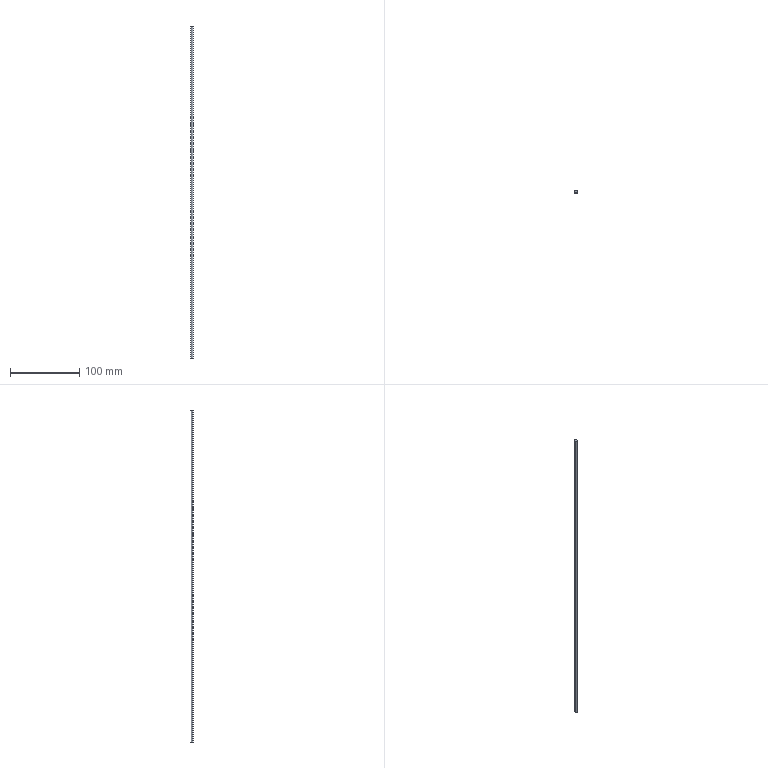Part | SolidWorks | features Extrusion 1 | 1 solid | 4 faces | box 4 x 4 x 479.4 mm | volume 6024 mm3 | cylinder 2 | plane 2 | commonest cylinder face diameters 4 x2
STEP:
#1=CARTESIAN_POINT('',(2.,0.,479.4));
#2=VERTEX_POINT('',#1);
#3=CARTESIAN_POINT('',(-2.,0.,479.4));
#4=VERTEX_POINT('',#3);
#5=CARTESIAN_POINT('',(0.,0.,479.4));
#6=DIRECTION('',(0.,0.,1.));
#7=DIRECTION('',(1.,0.,0.));
#8=AXIS2_PLACEMENT_3D('',#5,#6,#7);
#9=CIRCLE('',#8,2.);
#10=EDGE_CURVE('',#2,#4,#9,.T.);
#11=ORIENTED_EDGE('',*,*,#10,.F.);
#12=CARTESIAN_POINT('',(2.,0.,0.));
#13=VERTEX_POINT('',#12);
#14=CARTESIAN_POINT('',(2.,0.,479.4));
#15=DIRECTION('',(0.,0.,-1.));
#16=VECTOR('',#15,1000.);
#17=LINE('',#14,#16);
#18=EDGE_CURVE('',#2,#13,#17,.T.);
#19=ORIENTED_EDGE('',*,*,#18,.T.);
#20=CARTESIAN_POINT('',(-2.,0.,0.));
#21=VERTEX_POINT('',#20);
#22=CARTESIAN_POINT('',(0.,0.,0.));
#23=DIRECTION('',(0.,0.,1.));
#24=DIRECTION('',(1.,0.,0.));
#25=AXIS2_PLACEMENT_3D('',#22,#23,#24);
#26=CIRCLE('',#25,2.);
#27=EDGE_CURVE('',#13,#21,#26,.T.);
#28=ORIENTED_EDGE('',*,*,#27,.T.);
#29=CARTESIAN_POINT('',(-2.,0.,479.4));
#30=DIRECTION('',(0.,0.,-1.));
#31=VECTOR('',#30,1000.);
#32=LINE('',#29,#31);
#33=EDGE_CURVE('',#4,#21,#32,.T.);
#34=ORIENTED_EDGE('',*,*,#33,.F.);
#35=EDGE_LOOP('',(#11,#19,#28,#34));
#36=FACE_OUTER_BOUND('',#35,.T.);
#37=CARTESIAN_POINT('',(0.,0.,479.4));
#38=DIRECTION('',(0.,0.,-1.));
#39=DIRECTION('',(-1.,0.,0.));
#40=AXIS2_PLACEMENT_3D('',#37,#38,#39);
#41=CYLINDRICAL_SURFACE('',#40,2.);
#42=ADVANCED_FACE('',(#36),#41,.T.);
#43=ORIENTED_EDGE('',*,*,#18,.F.);
#44=CARTESIAN_POINT('',(0.,0.,479.4));
#45=DIRECTION('',(0.,0.,1.));
#46=DIRECTION('',(1.,0.,0.));
#47=AXIS2_PLACEMENT_3D('',#44,#45,#46);
#48=CIRCLE('',#47,2.);
#49=EDGE_CURVE('',#4,#2,#48,.T.);
#50=ORIENTED_EDGE('',*,*,#49,.F.);
#51=ORIENTED_EDGE('',*,*,#33,.T.);
#52=CARTESIAN_POINT('',(0.,0.,0.));
#53=DIRECTION('',(0.,0.,1.));
#54=DIRECTION('',(1.,0.,0.));
#55=AXIS2_PLACEMENT_3D('',#52,#53,#54);
#56=CIRCLE('',#55,2.);
#57=EDGE_CURVE('',#21,#13,#56,.T.);
#58=ORIENTED_EDGE('',*,*,#57,.T.);
#59=EDGE_LOOP('',(#43,#50,#51,#58));
#60=FACE_OUTER_BOUND('',#59,.T.);
#61=CARTESIAN_POINT('',(0.,0.,479.4));
#62=DIRECTION('',(0.,0.,-1.));
#63=DIRECTION('',(-1.,0.,0.));
#64=AXIS2_PLACEMENT_3D('',#61,#62,#63);
#65=CYLINDRICAL_SURFACE('',#64,2.);
#66=ADVANCED_FACE('',(#60),#65,.T.);
#67=ORIENTED_EDGE('',*,*,#49,.T.);
#68=ORIENTED_EDGE('',*,*,#10,.T.);
#69=EDGE_LOOP('',(#67,#68));
#70=FACE_OUTER_BOUND('',#69,.T.);
#71=CARTESIAN_POINT('',(0.,0.,479.4));
#72=DIRECTION('',(0.,0.,1.));
#73=DIRECTION('',(1.,0.,0.));
#74=AXIS2_PLACEMENT_3D('',#71,#72,#73);
#75=PLANE('',#74);
#76=ADVANCED_FACE('',(#70),#75,.T.);
#77=ORIENTED_EDGE('',*,*,#57,.F.);
#78=ORIENTED_EDGE('',*,*,#27,.F.);
#79=EDGE_LOOP('',(#77,#78));
#80=FACE_OUTER_BOUND('',#79,.T.);
#81=CARTESIAN_POINT('',(0.,0.,0.));
#82=DIRECTION('',(0.,0.,1.));
#83=DIRECTION('',(1.,0.,0.));
#84=AXIS2_PLACEMENT_3D('',#81,#82,#83);
#85=PLANE('',#84);
#86=ADVANCED_FACE('',(#80),#85,.F.);
#87=CLOSED_SHELL('',(#42,#66,#76,#86));
#88=MANIFOLD_SOLID_BREP('',#87);
#89=CARTESIAN_POINT('',(0.,0.,0.));
#90=DIRECTION('',(0.,0.,1.));
#91=DIRECTION('',(1.,0.,0.));
#92=AXIS2_PLACEMENT_3D('',#89,#90,#91);
#93=(LENGTH_UNIT()NAMED_UNIT(*)SI_UNIT(.MILLI.,.METRE.));
#94=UNCERTAINTY_MEASURE_WITH_UNIT(LENGTH_MEASURE(0.00001),#93,'','');
#95=(NAMED_UNIT(*)PLANE_ANGLE_UNIT()SI_UNIT($,.RADIAN.));
#96=(NAMED_UNIT(*)SI_UNIT($,.STERADIAN.)SOLID_ANGLE_UNIT());
#97=(GEOMETRIC_REPRESENTATION_CONTEXT(3)GLOBAL_UNCERTAINTY_ASSIGNED_CONTEXT((#94))GLOBAL_UNIT_ASSIGNED_CONTEXT((#93,#95,#96))REPRESENTATION_CONTEXT('',''));
#98=ADVANCED_BREP_SHAPE_REPRESENTATION('',(#88,#92),#97);